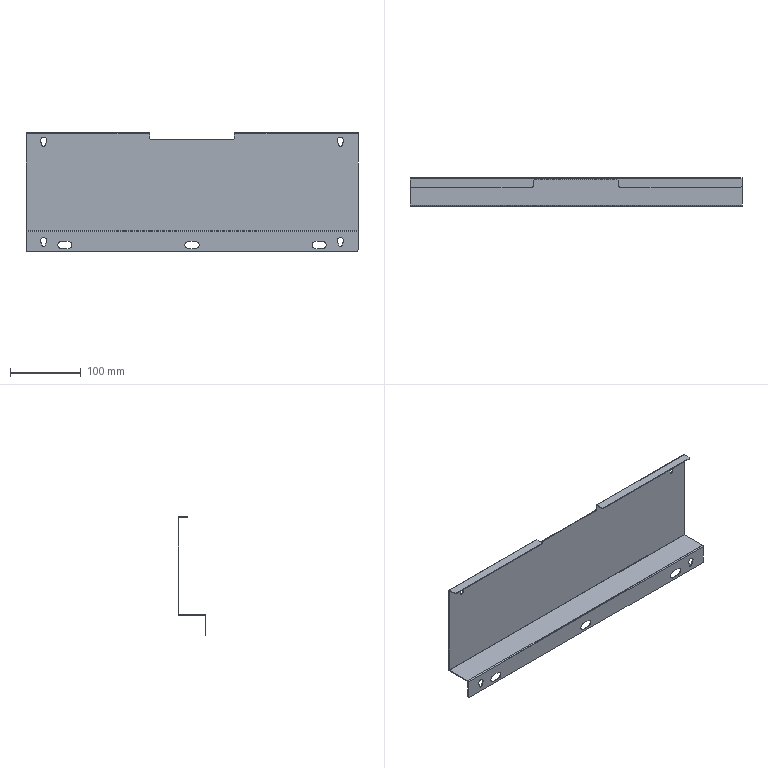Part | STEP file | 1 solid | 74 faces | box 470 x 39.5 x 167.8 mm | volume 118270 mm3 | plane 44 | cylinder 30 | commonest cylinder face diameters 4 x6 11 x6 0.4 x4 2.8 x4 5 x4 9 x4